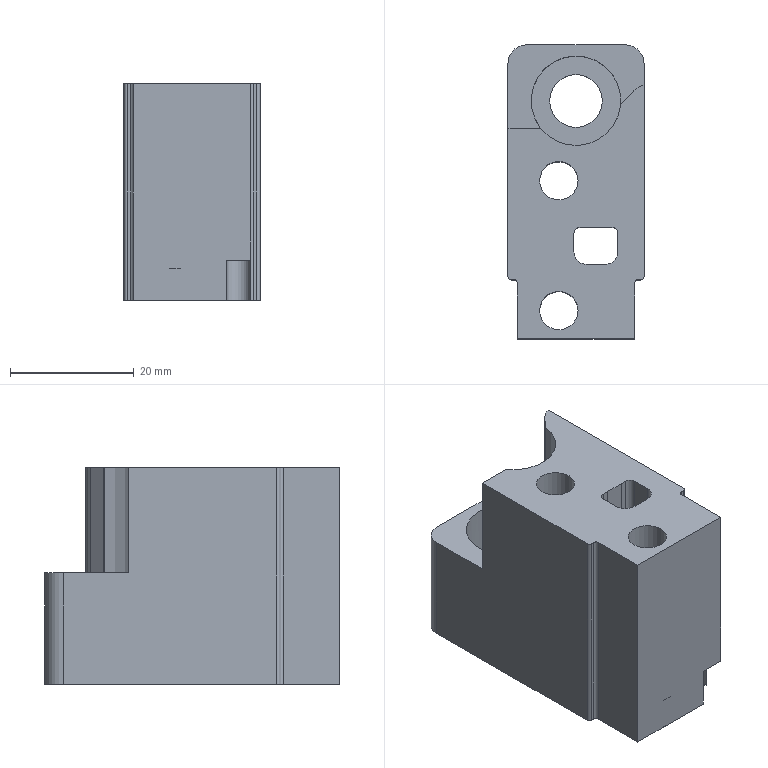Part | NX | features DIE-98 2 | 1 solid | 47 faces | box 22 x 47.549 x 35 mm | volume 24498 mm3 | plane 26 | cylinder 21 | commonest cylinder face diameters 6 x5 1 x4 4 x3 2 x2 6.2 x2 9 x2
STEP:
#1=CARTESIAN_POINT('',(4181.287,-820.122,858.716));
#2=VERTEX_POINT('',#1);
#3=CARTESIAN_POINT('',(4194.237,-816.266,858.716));
#4=VERTEX_POINT('',#3);
#5=CARTESIAN_POINT('',(4187.011,-815.672,858.716));
#6=DIRECTION('',(0.,0.,1.));
#7=DIRECTION('',(1.,0.,0.));
#8=AXIS2_PLACEMENT_3D('',#5,#6,#7);
#9=CIRCLE('',#8,7.25);
#10=EDGE_CURVE('',#2,#4,#9,.T.);
#11=ORIENTED_EDGE('',*,*,#10,.F.);
#12=CARTESIAN_POINT('',(4176.011,-820.122,858.716));
#13=VERTEX_POINT('',#12);
#14=CARTESIAN_POINT('',(3445.094,-820.122,858.716));
#15=DIRECTION('',(-1.,0.,0.));
#16=VECTOR('',#15,1000.);
#17=LINE('',#14,#16);
#18=EDGE_CURVE('',#2,#13,#17,.T.);
#19=ORIENTED_EDGE('',*,*,#18,.T.);
#20=CARTESIAN_POINT('',(4176.011,-844.123,858.716));
#21=VERTEX_POINT('',#20);
#22=CARTESIAN_POINT('',(4176.011,-999.122,858.716));
#23=DIRECTION('',(0.,-1.,0.));
#24=VECTOR('',#23,1000.);
#25=LINE('',#22,#24);
#26=EDGE_CURVE('',#13,#21,#25,.T.);
#27=ORIENTED_EDGE('',*,*,#26,.T.);
#28=CARTESIAN_POINT('',(4176.511,-844.623,858.716));
#29=VERTEX_POINT('',#28);
#30=CARTESIAN_POINT('',(4176.511,-844.123,858.716));
#31=DIRECTION('',(0.,0.,1.));
#32=DIRECTION('',(1.,0.,0.));
#33=AXIS2_PLACEMENT_3D('',#30,#31,#32);
#34=CIRCLE('',#33,0.5);
#35=EDGE_CURVE('',#21,#29,#34,.T.);
#36=ORIENTED_EDGE('',*,*,#35,.T.);
#37=CARTESIAN_POINT('',(4177.011,-844.623,858.716));
#38=VERTEX_POINT('',#37);
#39=CARTESIAN_POINT('',(3445.094,-844.623,858.716));
#40=DIRECTION('',(-1.,0.,0.));
#41=VECTOR('',#40,1000.);
#42=LINE('',#39,#41);
#43=EDGE_CURVE('',#29,#38,#42,.F.);
#44=ORIENTED_EDGE('',*,*,#43,.T.);
#45=CARTESIAN_POINT('',(4177.511,-845.123,858.716));
#46=VERTEX_POINT('',#45);
#47=CARTESIAN_POINT('',(4177.011,-845.123,858.716));
#48=DIRECTION('',(0.,0.,1.));
#49=DIRECTION('',(1.,0.,0.));
#50=AXIS2_PLACEMENT_3D('',#47,#48,#49);
#51=CIRCLE('',#50,0.5);
#52=EDGE_CURVE('',#38,#46,#51,.F.);
#53=ORIENTED_EDGE('',*,*,#52,.T.);
#54=CARTESIAN_POINT('',(4177.511,-854.172,858.716));
#55=VERTEX_POINT('',#54);
#56=CARTESIAN_POINT('',(4177.511,-839.123,858.716));
#57=DIRECTION('',(0.,-1.,0.));
#58=VECTOR('',#57,1000.);
#59=LINE('',#56,#58);
#60=EDGE_CURVE('',#46,#55,#59,.T.);
#61=ORIENTED_EDGE('',*,*,#60,.T.);
#62=CARTESIAN_POINT('',(4196.511,-854.172,858.716));
#63=VERTEX_POINT('',#62);
#64=CARTESIAN_POINT('',(4199.495,-854.172,858.716));
#65=DIRECTION('',(-1.,0.,0.));
#66=VECTOR('',#65,1000.);
#67=LINE('',#64,#66);
#68=EDGE_CURVE('',#63,#55,#67,.T.);
#69=ORIENTED_EDGE('',*,*,#68,.F.);
#70=CARTESIAN_POINT('',(4196.511,-845.123,858.716));
#71=VERTEX_POINT('',#70);
#72=CARTESIAN_POINT('',(4196.511,-839.123,858.716));
#73=DIRECTION('',(0.,1.,0.));
#74=VECTOR('',#73,1000.);
#75=LINE('',#72,#74);
#76=EDGE_CURVE('',#71,#63,#75,.F.);
#77=ORIENTED_EDGE('',*,*,#76,.F.);
#78=CARTESIAN_POINT('',(4197.011,-844.623,858.716));
#79=VERTEX_POINT('',#78);
#80=CARTESIAN_POINT('',(4197.011,-845.123,858.716));
#81=DIRECTION('',(0.,0.,1.));
#82=DIRECTION('',(1.,0.,0.));
#83=AXIS2_PLACEMENT_3D('',#80,#81,#82);
#84=CIRCLE('',#83,0.5);
#85=EDGE_CURVE('',#71,#79,#84,.F.);
#86=ORIENTED_EDGE('',*,*,#85,.T.);
#87=CARTESIAN_POINT('',(4197.511,-844.623,858.716));
#88=VERTEX_POINT('',#87);
#89=CARTESIAN_POINT('',(3445.094,-844.623,858.716));
#90=DIRECTION('',(-1.,0.,0.));
#91=VECTOR('',#90,1000.);
#92=LINE('',#89,#91);
#93=EDGE_CURVE('',#79,#88,#92,.F.);
#94=ORIENTED_EDGE('',*,*,#93,.T.);
#95=CARTESIAN_POINT('',(4198.011,-844.123,858.716));
#96=VERTEX_POINT('',#95);
#97=CARTESIAN_POINT('',(4197.511,-844.123,858.716));
#98=DIRECTION('',(0.,0.,1.));
#99=DIRECTION('',(1.,0.,0.));
#100=AXIS2_PLACEMENT_3D('',#97,#98,#99);
#101=CIRCLE('',#100,0.5);
#102=EDGE_CURVE('',#88,#96,#101,.T.);
#103=ORIENTED_EDGE('',*,*,#102,.T.);
#104=CARTESIAN_POINT('',(4198.011,-813.17,858.716));
#105=VERTEX_POINT('',#104);
#106=CARTESIAN_POINT('',(4198.011,-839.123,858.716));
#107=DIRECTION('',(0.,-1.,0.));
#108=VECTOR('',#107,1000.);
#109=LINE('',#106,#108);
#110=EDGE_CURVE('',#105,#96,#109,.T.);
#111=ORIENTED_EDGE('',*,*,#110,.F.);
#112=CARTESIAN_POINT('',(4196.39,-814.038,858.716));
#113=VERTEX_POINT('',#112);
#114=CARTESIAN_POINT('',(4198.548,-816.122,858.716));
#115=DIRECTION('',(0.,0.,1.));
#116=DIRECTION('',(1.,0.,0.));
#117=AXIS2_PLACEMENT_3D('',#114,#115,#116);
#118=CIRCLE('',#117,3.);
#119=EDGE_CURVE('',#113,#105,#118,.F.);
#120=ORIENTED_EDGE('',*,*,#119,.F.);
#121=CARTESIAN_POINT('',(4194.348,-816.153,858.716));
#122=VERTEX_POINT('',#121);
#123=CARTESIAN_POINT('',(3741.364,-1285.228,858.716));
#124=DIRECTION('',(-0.6947,-0.7193,0.));
#125=VECTOR('',#124,1000.);
#126=LINE('',#123,#125);
#127=EDGE_CURVE('',#113,#122,#126,.T.);
#128=ORIENTED_EDGE('',*,*,#127,.T.);
#129=CARTESIAN_POINT('',(4184.996,-807.122,858.716));
#130=DIRECTION('',(0.,0.,1.));
#131=DIRECTION('',(1.,0.,0.));
#132=AXIS2_PLACEMENT_3D('',#129,#130,#131);
#133=CIRCLE('',#132,13.);
#134=EDGE_CURVE('',#4,#122,#133,.T.);
#135=ORIENTED_EDGE('',*,*,#134,.F.);
#136=EDGE_LOOP('',(#11,#19,#27,#36,#44,#53,#61,#69,#77,#86,#94,#103,#111,#120,#128,#135));
#137=FACE_BOUND('',#136,.T.);
#138=CARTESIAN_POINT('',(4193.786,-837.122,858.716));
#139=VERTEX_POINT('',#138);
#140=CARTESIAN_POINT('',(4193.786,-840.122,858.716));
#141=VERTEX_POINT('',#140);
#142=CARTESIAN_POINT('',(4193.786,-839.122,858.716));
#143=DIRECTION('',(0.,-1.,0.));
#144=VECTOR('',#143,1000.);
#145=LINE('',#142,#144);
#146=EDGE_CURVE('',#139,#141,#145,.T.);
#147=ORIENTED_EDGE('',*,*,#146,.T.);
#148=CARTESIAN_POINT('',(4191.786,-842.122,858.716));
#149=VERTEX_POINT('',#148);
#150=CARTESIAN_POINT('',(4191.786,-840.122,858.716));
#151=DIRECTION('',(0.,0.,1.));
#152=DIRECTION('',(1.,0.,0.));
#153=AXIS2_PLACEMENT_3D('',#150,#151,#152);
#154=CIRCLE('',#153,2.);
#155=EDGE_CURVE('',#149,#141,#154,.T.);
#156=ORIENTED_EDGE('',*,*,#155,.F.);
#157=CARTESIAN_POINT('',(4188.686,-842.122,858.716));
#158=VERTEX_POINT('',#157);
#159=CARTESIAN_POINT('',(3445.094,-842.122,858.716));
#160=DIRECTION('',(1.,0.,0.));
#161=VECTOR('',#160,1000.);
#162=LINE('',#159,#161);
#163=EDGE_CURVE('',#158,#149,#162,.T.);
#164=ORIENTED_EDGE('',*,*,#163,.F.);
#165=CARTESIAN_POINT('',(4186.686,-840.122,858.716));
#166=VERTEX_POINT('',#165);
#167=CARTESIAN_POINT('',(4188.686,-840.122,858.716));
#168=DIRECTION('',(0.,0.,1.));
#169=DIRECTION('',(1.,0.,0.));
#170=AXIS2_PLACEMENT_3D('',#167,#168,#169);
#171=CIRCLE('',#170,2.);
#172=EDGE_CURVE('',#166,#158,#171,.T.);
#173=ORIENTED_EDGE('',*,*,#172,.F.);
#174=CARTESIAN_POINT('',(4186.686,-837.122,858.716));
#175=VERTEX_POINT('',#174);
#176=CARTESIAN_POINT('',(4186.686,-839.122,858.716));
#177=DIRECTION('',(0.,1.,0.));
#178=VECTOR('',#177,1000.);
#179=LINE('',#176,#178);
#180=EDGE_CURVE('',#166,#175,#179,.T.);
#181=ORIENTED_EDGE('',*,*,#180,.T.);
#182=CARTESIAN_POINT('',(4187.686,-836.122,858.716));
#183=VERTEX_POINT('',#182);
#184=CARTESIAN_POINT('',(4187.686,-837.122,858.716));
#185=DIRECTION('',(0.,0.,1.));
#186=DIRECTION('',(1.,0.,0.));
#187=AXIS2_PLACEMENT_3D('',#184,#185,#186);
#188=CIRCLE('',#187,1.);
#189=EDGE_CURVE('',#175,#183,#188,.F.);
#190=ORIENTED_EDGE('',*,*,#189,.T.);
#191=CARTESIAN_POINT('',(4188.686,-836.122,858.716));
#192=VERTEX_POINT('',#191);
#193=CARTESIAN_POINT('',(4190.736,-836.122,858.716));
#194=DIRECTION('',(1.,0.,0.));
#195=VECTOR('',#194,1000.);
#196=LINE('',#193,#195);
#197=EDGE_CURVE('',#183,#192,#196,.T.);
#198=ORIENTED_EDGE('',*,*,#197,.T.);
#199=CARTESIAN_POINT('',(4191.786,-836.122,858.716));
#200=VERTEX_POINT('',#199);
#201=CARTESIAN_POINT('',(4189.736,-836.122,858.716));
#202=DIRECTION('',(1.,0.,0.));
#203=VECTOR('',#202,1000.);
#204=LINE('',#201,#203);
#205=EDGE_CURVE('',#192,#200,#204,.T.);
#206=ORIENTED_EDGE('',*,*,#205,.T.);
#207=CARTESIAN_POINT('',(4192.786,-836.122,858.716));
#208=VERTEX_POINT('',#207);
#209=CARTESIAN_POINT('',(4190.736,-836.122,858.716));
#210=DIRECTION('',(1.,0.,0.));
#211=VECTOR('',#210,1000.);
#212=LINE('',#209,#211);
#213=EDGE_CURVE('',#200,#208,#212,.T.);
#214=ORIENTED_EDGE('',*,*,#213,.T.);
#215=CARTESIAN_POINT('',(4192.786,-837.122,858.716));
#216=DIRECTION('',(0.,0.,1.));
#217=DIRECTION('',(1.,0.,0.));
#218=AXIS2_PLACEMENT_3D('',#215,#216,#217);
#219=CIRCLE('',#218,1.);
#220=EDGE_CURVE('',#208,#139,#219,.F.);
#221=ORIENTED_EDGE('',*,*,#220,.T.);
#222=EDGE_LOOP('',(#147,#156,#164,#173,#181,#190,#198,#206,#214,#221));
#223=FACE_BOUND('',#222,.T.);
#224=CARTESIAN_POINT('',(4187.336,-828.622,858.716));
#225=VERTEX_POINT('',#224);
#226=CARTESIAN_POINT('',(4184.236,-828.622,858.716));
#227=DIRECTION('',(0.,0.,1.));
#228=DIRECTION('',(1.,0.,0.));
#229=AXIS2_PLACEMENT_3D('',#226,#227,#228);
#230=CIRCLE('',#229,3.1);
#231=EDGE_CURVE('',#225,#225,#230,.F.);
#232=ORIENTED_EDGE('',*,*,#231,.T.);
#233=EDGE_LOOP('',(#232));
#234=FACE_BOUND('',#233,.T.);
#235=CARTESIAN_POINT('',(4187.336,-849.622,858.716));
#236=VERTEX_POINT('',#235);
#237=CARTESIAN_POINT('',(4184.236,-849.622,858.716));
#238=DIRECTION('',(0.,0.,1.));
#239=DIRECTION('',(1.,0.,0.));
#240=AXIS2_PLACEMENT_3D('',#237,#238,#239);
#241=CIRCLE('',#240,3.1);
#242=EDGE_CURVE('',#236,#236,#241,.T.);
#243=ORIENTED_EDGE('',*,*,#242,.F.);
#244=EDGE_LOOP('',(#243));
#245=FACE_BOUND('',#244,.T.);
#246=CARTESIAN_POINT('',(3445.094,-999.122,858.716));
#247=DIRECTION('',(0.,0.,1.));
#248=DIRECTION('',(0.,1.,0.));
#249=AXIS2_PLACEMENT_3D('',#246,#247,#248);
#250=PLANE('',#249);
#251=ADVANCED_FACE('',(#137,#223,#234,#245),#250,.T.);
#252=ORIENTED_EDGE('',*,*,#26,.F.);
#253=CARTESIAN_POINT('',(4176.011,-820.122,841.716));
#254=VERTEX_POINT('',#253);
#255=CARTESIAN_POINT('',(4176.011,-820.122,823.716));
#256=DIRECTION('',(0.,0.,-1.));
#257=VECTOR('',#256,1000.);
#258=LINE('',#255,#257);
#259=EDGE_CURVE('',#13,#254,#258,.T.);
#260=ORIENTED_EDGE('',*,*,#259,.T.);
#261=CARTESIAN_POINT('',(4176.011,-809.623,841.716));
#262=VERTEX_POINT('',#261);
#263=CARTESIAN_POINT('',(4176.011,-813.754,841.716));
#264=DIRECTION('',(0.,1.,0.));
#265=VECTOR('',#264,1000.);
#266=LINE('',#263,#265);
#267=EDGE_CURVE('',#262,#254,#266,.F.);
#268=ORIENTED_EDGE('',*,*,#267,.F.);
#269=CARTESIAN_POINT('',(4176.011,-809.623,823.716));
#270=VERTEX_POINT('',#269);
#271=CARTESIAN_POINT('',(4176.011,-809.623,823.716));
#272=DIRECTION('',(0.,0.,1.));
#273=VECTOR('',#272,1000.);
#274=LINE('',#271,#273);
#275=EDGE_CURVE('',#270,#262,#274,.T.);
#276=ORIENTED_EDGE('',*,*,#275,.F.);
#277=CARTESIAN_POINT('',(4176.011,-844.123,823.716));
#278=VERTEX_POINT('',#277);
#279=CARTESIAN_POINT('',(4176.011,-999.122,823.716));
#280=DIRECTION('',(0.,-1.,0.));
#281=VECTOR('',#280,1000.);
#282=LINE('',#279,#281);
#283=EDGE_CURVE('',#278,#270,#282,.F.);
#284=ORIENTED_EDGE('',*,*,#283,.F.);
#285=CARTESIAN_POINT('',(4176.011,-844.123,823.716));
#286=DIRECTION('',(0.,0.,1.));
#287=VECTOR('',#286,1000.);
#288=LINE('',#285,#287);
#289=EDGE_CURVE('',#278,#21,#288,.T.);
#290=ORIENTED_EDGE('',*,*,#289,.T.);
#291=EDGE_LOOP('',(#252,#260,#268,#276,#284,#290));
#292=FACE_BOUND('',#291,.T.);
#293=CARTESIAN_POINT('',(4176.011,-839.123,823.716));
#294=DIRECTION('',(-1.,0.,0.));
#295=DIRECTION('',(0.,0.,1.));
#296=AXIS2_PLACEMENT_3D('',#293,#294,#295);
#297=PLANE('',#296);
#298=ADVANCED_FACE('',(#292),#297,.T.);
#299=CARTESIAN_POINT('',(4191.261,-815.672,823.716));
#300=VERTEX_POINT('',#299);
#301=CARTESIAN_POINT('',(4187.011,-815.672,823.716));
#302=DIRECTION('',(0.,0.,1.));
#303=DIRECTION('',(1.,0.,0.));
#304=AXIS2_PLACEMENT_3D('',#301,#302,#303);
#305=CIRCLE('',#304,4.25);
#306=EDGE_CURVE('',#300,#300,#305,.F.);
#307=ORIENTED_EDGE('',*,*,#306,.F.);
#308=EDGE_LOOP('',(#307));
#309=FACE_BOUND('',#308,.T.);
#310=CARTESIAN_POINT('',(4186.686,-839.69,823.716));
#311=VERTEX_POINT('',#310);
#312=CARTESIAN_POINT('',(4188.236,-834.122,823.716));
#313=VERTEX_POINT('',#312);
#314=CARTESIAN_POINT('',(4188.236,-837.122,823.716));
#315=DIRECTION('',(0.,0.,1.));
#316=DIRECTION('',(1.,0.,0.));
#317=AXIS2_PLACEMENT_3D('',#314,#315,#316);
#318=CIRCLE('',#317,3.);
#319=EDGE_CURVE('',#311,#313,#318,.F.);
#320=ORIENTED_EDGE('',*,*,#319,.F.);
#321=CARTESIAN_POINT('',(4186.686,-840.122,823.716));
#322=VERTEX_POINT('',#321);
#323=CARTESIAN_POINT('',(4186.686,-839.122,823.716));
#324=DIRECTION('',(0.,1.,0.));
#325=VECTOR('',#324,1000.);
#326=LINE('',#323,#325);
#327=EDGE_CURVE('',#311,#322,#326,.F.);
#328=ORIENTED_EDGE('',*,*,#327,.T.);
#329=CARTESIAN_POINT('',(4188.686,-842.122,823.716));
#330=VERTEX_POINT('',#329);
#331=CARTESIAN_POINT('',(4188.686,-840.122,823.716));
#332=DIRECTION('',(0.,0.,1.));
#333=DIRECTION('',(1.,0.,0.));
#334=AXIS2_PLACEMENT_3D('',#331,#332,#333);
#335=CIRCLE('',#334,2.);
#336=EDGE_CURVE('',#330,#322,#335,.F.);
#337=ORIENTED_EDGE('',*,*,#336,.F.);
#338=CARTESIAN_POINT('',(4191.786,-842.122,823.716));
#339=VERTEX_POINT('',#338);
#340=CARTESIAN_POINT('',(3445.094,-842.122,823.716));
#341=DIRECTION('',(1.,0.,0.));
#342=VECTOR('',#341,1000.);
#343=LINE('',#340,#342);
#344=EDGE_CURVE('',#339,#330,#343,.F.);
#345=ORIENTED_EDGE('',*,*,#344,.F.);
#346=CARTESIAN_POINT('',(4193.786,-840.122,823.716));
#347=VERTEX_POINT('',#346);
#348=CARTESIAN_POINT('',(4191.786,-840.122,823.716));
#349=DIRECTION('',(0.,0.,1.));
#350=DIRECTION('',(1.,0.,0.));
#351=AXIS2_PLACEMENT_3D('',#348,#349,#350);
#352=CIRCLE('',#351,2.);
#353=EDGE_CURVE('',#347,#339,#352,.F.);
#354=ORIENTED_EDGE('',*,*,#353,.F.);
#355=CARTESIAN_POINT('',(4193.786,-839.69,823.716));
#356=VERTEX_POINT('',#355);
#357=CARTESIAN_POINT('',(4193.786,-839.122,823.716));
#358=DIRECTION('',(0.,-1.,0.));
#359=VECTOR('',#358,1000.);
#360=LINE('',#357,#359);
#361=EDGE_CURVE('',#347,#356,#360,.F.);
#362=ORIENTED_EDGE('',*,*,#361,.T.);
#363=CARTESIAN_POINT('',(4192.236,-834.122,823.716));
#364=VERTEX_POINT('',#363);
#365=CARTESIAN_POINT('',(4192.236,-837.122,823.716));
#366=DIRECTION('',(0.,0.,1.));
#367=DIRECTION('',(1.,0.,0.));
#368=AXIS2_PLACEMENT_3D('',#365,#366,#367);
#369=CIRCLE('',#368,3.);
#370=EDGE_CURVE('',#364,#356,#369,.F.);
#371=ORIENTED_EDGE('',*,*,#370,.F.);
#372=CARTESIAN_POINT('',(4188.236,-834.122,823.716));
#373=DIRECTION('',(-1.,0.,0.));
#374=VECTOR('',#373,1000.);
#375=LINE('',#372,#374);
#376=EDGE_CURVE('',#313,#364,#375,.F.);
#377=ORIENTED_EDGE('',*,*,#376,.F.);
#378=EDGE_LOOP('',(#320,#328,#337,#345,#354,#362,#371,#377));
#379=FACE_BOUND('',#378,.T.);
#380=CARTESIAN_POINT('',(4188.736,-828.622,823.716));
#381=VERTEX_POINT('',#380);
#382=CARTESIAN_POINT('',(4184.236,-828.622,823.716));
#383=DIRECTION('',(0.,0.,1.));
#384=DIRECTION('',(1.,0.,0.));
#385=AXIS2_PLACEMENT_3D('',#382,#383,#384);
#386=CIRCLE('',#385,4.5);
#387=EDGE_CURVE('',#381,#381,#386,.T.);
#388=ORIENTED_EDGE('',*,*,#387,.T.);
#389=EDGE_LOOP('',(#388));
#390=FACE_BOUND('',#389,.T.);
#391=CARTESIAN_POINT('',(4188.736,-849.622,823.716));
#392=VERTEX_POINT('',#391);
#393=CARTESIAN_POINT('',(4184.236,-849.622,823.716));
#394=DIRECTION('',(0.,0.,1.));
#395=DIRECTION('',(1.,0.,0.));
#396=AXIS2_PLACEMENT_3D('',#393,#394,#395);
#397=CIRCLE('',#396,4.5);
#398=EDGE_CURVE('',#392,#392,#397,.T.);
#399=ORIENTED_EDGE('',*,*,#398,.T.);
#400=EDGE_LOOP('',(#399));
#401=FACE_BOUND('',#400,.T.);
#402=CARTESIAN_POINT('',(4192.535,-851.122,823.716));
#403=VERTEX_POINT('',#402);
#404=CARTESIAN_POINT('',(4196.511,-850.812,823.716));
#405=VERTEX_POINT('',#404);
#406=CARTESIAN_POINT('',(4194.535,-851.122,823.716));
#407=DIRECTION('',(0.,0.,-1.));
#408=DIRECTION('',(1.,0.,0.));
#409=AXIS2_PLACEMENT_3D('',#406,#407,#408);
#410=CIRCLE('',#409,2.);
#411=EDGE_CURVE('',#403,#405,#410,.T.);
#412=ORIENTED_EDGE('',*,*,#411,.F.);
#413=CARTESIAN_POINT('',(4192.535,-854.172,823.716));
#414=VERTEX_POINT('',#413);
#415=CARTESIAN_POINT('',(4192.535,-851.122,823.716));
#416=DIRECTION('',(0.,-1.,0.));
#417=VECTOR('',#416,1000.);
#418=LINE('',#415,#417);
#419=EDGE_CURVE('',#403,#414,#418,.T.);
#420=ORIENTED_EDGE('',*,*,#419,.T.);
#421=CARTESIAN_POINT('',(4177.511,-854.172,823.716));
#422=VERTEX_POINT('',#421);
#423=CARTESIAN_POINT('',(3445.094,-854.172,823.716));
#424=DIRECTION('',(-1.,0.,0.));
#425=VECTOR('',#424,1000.);
#426=LINE('',#423,#425);
#427=EDGE_CURVE('',#422,#414,#426,.F.);
#428=ORIENTED_EDGE('',*,*,#427,.F.);
#429=CARTESIAN_POINT('',(4177.511,-845.123,823.716));
#430=VERTEX_POINT('',#429);
#431=CARTESIAN_POINT('',(4177.511,-839.123,823.716));
#432=DIRECTION('',(0.,1.,0.));
#433=VECTOR('',#432,1000.);
#434=LINE('',#431,#433);
#435=EDGE_CURVE('',#422,#430,#434,.T.);
#436=ORIENTED_EDGE('',*,*,#435,.T.);
#437=CARTESIAN_POINT('',(4177.011,-844.623,823.716));
#438=VERTEX_POINT('',#437);
#439=CARTESIAN_POINT('',(4177.011,-845.123,823.716));
#440=DIRECTION('',(0.,0.,1.));
#441=DIRECTION('',(1.,0.,0.));
#442=AXIS2_PLACEMENT_3D('',#439,#440,#441);
#443=CIRCLE('',#442,0.5);
#444=EDGE_CURVE('',#430,#438,#443,.T.);
#445=ORIENTED_EDGE('',*,*,#444,.T.);
#446=CARTESIAN_POINT('',(4176.511,-844.623,823.716));
#447=VERTEX_POINT('',#446);
#448=CARTESIAN_POINT('',(3445.094,-844.623,823.716));
#449=DIRECTION('',(-1.,0.,0.));
#450=VECTOR('',#449,1000.);
#451=LINE('',#448,#450);
#452=EDGE_CURVE('',#447,#438,#451,.F.);
#453=ORIENTED_EDGE('',*,*,#452,.F.);
#454=CARTESIAN_POINT('',(4176.511,-844.123,823.716));
#455=DIRECTION('',(0.,0.,1.));
#456=DIRECTION('',(1.,0.,0.));
#457=AXIS2_PLACEMENT_3D('',#454,#455,#456);
#458=CIRCLE('',#457,0.5);
#459=EDGE_CURVE('',#447,#278,#458,.F.);
#460=ORIENTED_EDGE('',*,*,#459,.T.);
#461=ORIENTED_EDGE('',*,*,#283,.T.);
#462=CARTESIAN_POINT('',(4179.011,-806.623,823.716));
#463=VERTEX_POINT('',#462);
#464=CARTESIAN_POINT('',(4179.011,-809.623,823.716));
#465=DIRECTION('',(0.,0.,1.));
#466=DIRECTION('',(-1.,0.,0.));
#467=AXIS2_PLACEMENT_3D('',#464,#465,#466);
#468=CIRCLE('',#467,3.);
#469=EDGE_CURVE('',#463,#270,#468,.T.);
#470=ORIENTED_EDGE('',*,*,#469,.F.);
#471=CARTESIAN_POINT('',(4195.011,-806.623,823.716));
#472=VERTEX_POINT('',#471);
#473=CARTESIAN_POINT('',(3445.094,-806.623,823.716));
#474=DIRECTION('',(-1.,0.,0.));
#475=VECTOR('',#474,1000.);
#476=LINE('',#473,#475);
#477=EDGE_CURVE('',#463,#472,#476,.F.);
#478=ORIENTED_EDGE('',*,*,#477,.T.);
#479=CARTESIAN_POINT('',(4198.011,-809.623,823.716));
#480=VERTEX_POINT('',#479);
#481=CARTESIAN_POINT('',(4195.011,-809.623,823.716));
#482=DIRECTION('',(0.,0.,1.));
#483=DIRECTION('',(-1.,0.,0.));
#484=AXIS2_PLACEMENT_3D('',#481,#482,#483);
#485=CIRCLE('',#484,3.);
#486=EDGE_CURVE('',#480,#472,#485,.T.);
#487=ORIENTED_EDGE('',*,*,#486,.F.);
#488=CARTESIAN_POINT('',(4198.011,-844.123,823.716));
#489=VERTEX_POINT('',#488);
#490=CARTESIAN_POINT('',(4198.011,-999.122,823.716));
#491=DIRECTION('',(0.,1.,0.));
#492=VECTOR('',#491,1000.);
#493=LINE('',#490,#492);
#494=EDGE_CURVE('',#480,#489,#493,.F.);
#495=ORIENTED_EDGE('',*,*,#494,.T.);
#496=CARTESIAN_POINT('',(4197.511,-844.623,823.716));
#497=VERTEX_POINT('',#496);
#498=CARTESIAN_POINT('',(4197.511,-844.123,823.716));
#499=DIRECTION('',(0.,0.,1.));
#500=DIRECTION('',(1.,0.,0.));
#501=AXIS2_PLACEMENT_3D('',#498,#499,#500);
#502=CIRCLE('',#501,0.5);
#503=EDGE_CURVE('',#489,#497,#502,.F.);
#504=ORIENTED_EDGE('',*,*,#503,.T.);
#505=CARTESIAN_POINT('',(4197.011,-844.623,823.716));
#506=VERTEX_POINT('',#505);
#507=CARTESIAN_POINT('',(3445.094,-844.623,823.716));
#508=DIRECTION('',(-1.,0.,0.));
#509=VECTOR('',#508,1000.);
#510=LINE('',#507,#509);
#511=EDGE_CURVE('',#506,#497,#510,.F.);
#512=ORIENTED_EDGE('',*,*,#511,.F.);
#513=CARTESIAN_POINT('',(4196.511,-845.123,823.716));
#514=VERTEX_POINT('',#513);
#515=CARTESIAN_POINT('',(4197.011,-845.123,823.716));
#516=DIRECTION('',(0.,0.,1.));
#517=DIRECTION('',(1.,0.,0.));
#518=AXIS2_PLACEMENT_3D('',#515,#516,#517);
#519=CIRCLE('',#518,0.5);
#520=EDGE_CURVE('',#506,#514,#519,.T.);
#521=ORIENTED_EDGE('',*,*,#520,.T.);
#522=CARTESIAN_POINT('',(4196.511,-839.123,823.716));
#523=DIRECTION('',(0.,-1.,0.));
#524=VECTOR('',#523,1000.);
#525=LINE('',#522,#524);
#526=EDGE_CURVE('',#514,#405,#525,.T.);
#527=ORIENTED_EDGE('',*,*,#526,.T.);
#528=EDGE_LOOP('',(#412,#420,#428,#436,#445,#453,#460,#461,#470,#478,#487,#495,#504,#512,#521,#527));
#529=FACE_BOUND('',#528,.T.);
#530=CARTESIAN_POINT('',(3445.094,-999.122,823.716));
#531=DIRECTION('',(0.,0.,1.));
#532=DIRECTION('',(0.,1.,0.));
#533=AXIS2_PLACEMENT_3D('',#530,#531,#532);
#534=PLANE('',#533);
#535=ADVANCED_FACE('',(#309,#379,#390,#401,#529),#534,.F.);
#536=CARTESIAN_POINT('',(4192.535,-854.172,830.216));
#537=VERTEX_POINT('',#536);
#538=CARTESIAN_POINT('',(4192.535,-854.172,858.716));
#539=DIRECTION('',(0.,0.,-1.));
#540=VECTOR('',#539,1000.);
#541=LINE('',#538,#540);
#542=EDGE_CURVE('',#537,#414,#541,.T.);
#543=ORIENTED_EDGE('',*,*,#542,.F.);
#544=CARTESIAN_POINT('',(4196.511,-854.172,830.216));
#545=VERTEX_POINT('',#544);
#546=CARTESIAN_POINT('',(4199.495,-854.172,830.216));
#547=DIRECTION('',(-1.,0.,0.));
#548=VECTOR('',#547,1000.);
#549=LINE('',#546,#548);
#550=EDGE_CURVE('',#545,#537,#549,.T.);
#551=ORIENTED_EDGE('',*,*,#550,.F.);
#552=CARTESIAN_POINT('',(4196.511,-854.172,858.716));
#553=DIRECTION('',(0.,0.,-1.));
#554=VECTOR('',#553,1000.);
#555=LINE('',#552,#554);
#556=EDGE_CURVE('',#63,#545,#555,.T.);
#557=ORIENTED_EDGE('',*,*,#556,.F.);
#558=ORIENTED_EDGE('',*,*,#68,.T.);
#559=CARTESIAN_POINT('',(4177.511,-854.172,823.716));
#560=DIRECTION('',(0.,0.,-1.));
#561=VECTOR('',#560,1000.);
#562=LINE('',#559,#561);
#563=EDGE_CURVE('',#55,#422,#562,.T.);
#564=ORIENTED_EDGE('',*,*,#563,.T.);
#565=ORIENTED_EDGE('',*,*,#427,.T.);
#566=EDGE_LOOP('',(#543,#551,#557,#558,#564,#565));
#567=FACE_BOUND('',#566,.T.);
#568=CARTESIAN_POINT('',(4199.495,-854.172,858.716));
#569=DIRECTION('',(0.,1.,0.));
#570=DIRECTION('',(-1.,0.,0.));
#571=AXIS2_PLACEMENT_3D('',#568,#569,#570);
#572=PLANE('',#571);
#573=ADVANCED_FACE('',(#567),#572,.F.);
#574=ORIENTED_EDGE('',*,*,#511,.T.);
#575=CARTESIAN_POINT('',(4197.511,-844.623,858.716));
#576=DIRECTION('',(0.,0.,-1.));
#577=VECTOR('',#576,1000.);
#578=LINE('',#575,#577);
#579=EDGE_CURVE('',#497,#88,#578,.F.);
#580=ORIENTED_EDGE('',*,*,#579,.T.);
#581=ORIENTED_EDGE('',*,*,#93,.F.);
#582=CARTESIAN_POINT('',(4197.011,-844.623,841.216));
#583=DIRECTION('',(0.,0.,1.));
#584=VECTOR('',#583,1000.);
#585=LINE('',#582,#584);
#586=EDGE_CURVE('',#79,#506,#585,.F.);
#587=ORIENTED_EDGE('',*,*,#586,.T.);
#588=EDGE_LOOP('',(#574,#580,#581,#587));
#589=FACE_BOUND('',#588,.T.);
#590=CARTESIAN_POINT('',(4187.011,-844.623,841.216));
#591=DIRECTION('',(0.,1.,0.));
#592=DIRECTION('',(0.,0.,1.));
#593=AXIS2_PLACEMENT_3D('',#590,#591,#592);
#594=PLANE('',#593);
#595=ADVANCED_FACE('',(#589),#594,.F.);
#596=ORIENTED_EDGE('',*,*,#452,.T.);
#597=CARTESIAN_POINT('',(4177.011,-844.623,841.216));
#598=DIRECTION('',(0.,0.,-1.));
#599=VECTOR('',#598,1000.);
#600=LINE('',#597,#599);
#601=EDGE_CURVE('',#438,#38,#600,.F.);
#602=ORIENTED_EDGE('',*,*,#601,.T.);
#603=ORIENTED_EDGE('',*,*,#43,.F.);
#604=CARTESIAN_POINT('',(4176.511,-844.623,823.716));
#605=DIRECTION('',(0.,0.,1.));
#606=VECTOR('',#605,1000.);
#607=LINE('',#604,#606);
#608=EDGE_CURVE('',#29,#447,#607,.F.);
#609=ORIENTED_EDGE('',*,*,#608,.T.);
#610=EDGE_LOOP('',(#596,#602,#603,#609));
#611=FACE_BOUND('',#610,.T.);
#612=CARTESIAN_POINT('',(4187.011,-844.623,841.216));
#613=DIRECTION('',(0.,1.,0.));
#614=DIRECTION('',(0.,0.,1.));
#615=AXIS2_PLACEMENT_3D('',#612,#613,#614);
#616=PLANE('',#615);
#617=ADVANCED_FACE('',(#611),#616,.F.);
#618=CARTESIAN_POINT('',(4181.136,-828.622,828.916));
#619=VERTEX_POINT('',#618);
#620=CARTESIAN_POINT('',(4184.236,-828.622,828.916));
#621=DIRECTION('',(0.,0.,-1.));
#622=DIRECTION('',(-1.,0.,0.));
#623=AXIS2_PLACEMENT_3D('',#620,#621,#622);
#624=CIRCLE('',#623,3.1);
#625=EDGE_CURVE('',#619,#619,#624,.T.);
#626=ORIENTED_EDGE('',*,*,#625,.F.);
#627=EDGE_LOOP('',(#626));
#628=FACE_BOUND('',#627,.T.);
#629=CARTESIAN_POINT('',(4179.736,-828.622,828.916));
#630=VERTEX_POINT('',#629);
#631=CARTESIAN_POINT('',(4184.236,-828.622,828.916));
#632=DIRECTION('',(0.,0.,-1.));
#633=DIRECTION('',(-1.,0.,0.));
#634=AXIS2_PLACEMENT_3D('',#631,#632,#633);
#635=CIRCLE('',#634,4.5);
#636=EDGE_CURVE('',#630,#630,#635,.F.);
#637=ORIENTED_EDGE('',*,*,#636,.F.);
#638=EDGE_LOOP('',(#637));
#639=FACE_BOUND('',#638,.T.);
#640=CARTESIAN_POINT('',(4217.236,-877.122,828.916));
#641=DIRECTION('',(0.,0.,-1.));
#642=DIRECTION('',(-1.,0.,0.));
#643=AXIS2_PLACEMENT_3D('',#640,#641,#642);
#644=PLANE('',#643);
#645=ADVANCED_FACE('',(#628,#639),#644,.T.);
#646=CARTESIAN_POINT('',(4186.686,-839.69,828.916));
#647=VERTEX_POINT('',#646);
#648=CARTESIAN_POINT('',(4186.686,-837.122,828.916));
#649=VERTEX_POINT('',#648);
#650=CARTESIAN_POINT('',(4186.686,-1716.244,828.916));
#651=DIRECTION('',(0.,1.,0.));
#652=VECTOR('',#651,1000.);
#653=LINE('',#650,#652);
#654=EDGE_CURVE('',#647,#649,#653,.T.);
#655=ORIENTED_EDGE('',*,*,#654,.F.);
#656=CARTESIAN_POINT('',(4188.236,-834.122,828.916));
#657=VERTEX_POINT('',#656);
#658=CARTESIAN_POINT('',(4188.236,-837.122,828.916));
#659=DIRECTION('',(0.,0.,-1.));
#660=DIRECTION('',(-1.,0.,0.));
#661=AXIS2_PLACEMENT_3D('',#658,#659,#660);
#662=CIRCLE('',#661,3.);
#663=EDGE_CURVE('',#647,#657,#662,.T.);
#664=ORIENTED_EDGE('',*,*,#663,.T.);
#665=CARTESIAN_POINT('',(4192.236,-834.122,828.916));
#666=VERTEX_POINT('',#665);
#667=CARTESIAN_POINT('',(4188.236,-834.122,828.916));
#668=DIRECTION('',(1.,0.,0.));
#669=VECTOR('',#668,1000.);
#670=LINE('',#667,#669);
#671=EDGE_CURVE('',#657,#666,#670,.T.);
#672=ORIENTED_EDGE('',*,*,#671,.T.);
#673=CARTESIAN_POINT('',(4193.786,-839.69,828.916));
#674=VERTEX_POINT('',#673);
#675=CARTESIAN_POINT('',(4192.236,-837.122,828.916));
#676=DIRECTION('',(0.,0.,-1.));
#677=DIRECTION('',(-1.,0.,0.));
#678=AXIS2_PLACEMENT_3D('',#675,#676,#677);
#679=CIRCLE('',#678,3.);
#680=EDGE_CURVE('',#666,#674,#679,.T.);
#681=ORIENTED_EDGE('',*,*,#680,.T.);
#682=CARTESIAN_POINT('',(4193.786,-837.122,828.916));
#683=VERTEX_POINT('',#682);
#684=CARTESIAN_POINT('',(4193.786,-1716.244,828.916));
#685=DIRECTION('',(0.,-1.,0.));
#686=VECTOR('',#685,1000.);
#687=LINE('',#684,#686);
#688=EDGE_CURVE('',#683,#674,#687,.T.);
#689=ORIENTED_EDGE('',*,*,#688,.F.);
#690=CARTESIAN_POINT('',(4192.786,-836.122,828.916));
#691=VERTEX_POINT('',#690);
#692=CARTESIAN_POINT('',(4192.786,-837.122,828.916));
#693=DIRECTION('',(0.,0.,-1.));
#694=DIRECTION('',(-1.,0.,0.));
#695=AXIS2_PLACEMENT_3D('',#692,#693,#694);
#696=CIRCLE('',#695,1.);
#697=EDGE_CURVE('',#691,#683,#696,.T.);
#698=ORIENTED_EDGE('',*,*,#697,.F.);
#699=CARTESIAN_POINT('',(4192.236,-836.122,828.916));
#700=VERTEX_POINT('',#699);
#701=CARTESIAN_POINT('',(4190.736,-836.122,828.916));
#702=DIRECTION('',(-1.,0.,0.));
#703=VECTOR('',#702,1000.);
#704=LINE('',#701,#703);
#705=EDGE_CURVE('',#691,#700,#704,.T.);
#706=ORIENTED_EDGE('',*,*,#705,.T.);
#707=CARTESIAN_POINT('',(4191.786,-836.122,828.916));
#708=VERTEX_POINT('',#707);
#709=CARTESIAN_POINT('',(4190.736,-836.122,828.916));
#710=DIRECTION('',(-1.,0.,0.));
#711=VECTOR('',#710,1000.);
#712=LINE('',#709,#711);
#713=EDGE_CURVE('',#700,#708,#712,.T.);
#714=ORIENTED_EDGE('',*,*,#713,.T.);
#715=CARTESIAN_POINT('',(4188.686,-836.122,828.916));
#716=VERTEX_POINT('',#715);
#717=CARTESIAN_POINT('',(0.000000109,-836.122,828.916));
#718=DIRECTION('',(1.,0.,0.));
#719=VECTOR('',#718,1000.);
#720=LINE('',#717,#719);
#721=EDGE_CURVE('',#716,#708,#720,.T.);
#722=ORIENTED_EDGE('',*,*,#721,.F.);
#723=CARTESIAN_POINT('',(4188.236,-836.122,828.916));
#724=VERTEX_POINT('',#723);
#725=CARTESIAN_POINT('',(4190.736,-836.122,828.916));
#726=DIRECTION('',(-1.,0.,0.));
#727=VECTOR('',#726,1000.);
#728=LINE('',#725,#727);
#729=EDGE_CURVE('',#716,#724,#728,.T.);
#730=ORIENTED_EDGE('',*,*,#729,.T.);
#731=CARTESIAN_POINT('',(4187.686,-836.122,828.916));
#732=VERTEX_POINT('',#731);
#733=CARTESIAN_POINT('',(4190.736,-836.122,828.916));
#734=DIRECTION('',(-1.,0.,0.));
#735=VECTOR('',#734,1000.);
#736=LINE('',#733,#735);
#737=EDGE_CURVE('',#724,#732,#736,.T.);
#738=ORIENTED_EDGE('',*,*,#737,.T.);
#739=CARTESIAN_POINT('',(4187.686,-837.122,828.916));
#740=DIRECTION('',(0.,0.,-1.));
#741=DIRECTION('',(-1.,0.,0.));
#742=AXIS2_PLACEMENT_3D('',#739,#740,#741);
#743=CIRCLE('',#742,1.);
#744=EDGE_CURVE('',#649,#732,#743,.T.);
#745=ORIENTED_EDGE('',*,*,#744,.F.);
#746=EDGE_LOOP('',(#655,#664,#672,#681,#689,#698,#706,#714,#722,#730,#738,#745));
#747=FACE_BOUND('',#746,.T.);
#748=CARTESIAN_POINT('',(0.000000011,-1716.244,828.916));
#749=DIRECTION('',(0.,0.,-1.));
#750=DIRECTION('',(-1.,0.,0.));
#751=AXIS2_PLACEMENT_3D('',#748,#749,#750);
#752=PLANE('',#751);
#753=ADVANCED_FACE('',(#747),#752,.T.);
#754=ORIENTED_EDGE('',*,*,#231,.F.);
#755=EDGE_LOOP('',(#754));
#756=FACE_BOUND('',#755,.T.);
#757=ORIENTED_EDGE('',*,*,#625,.T.);
#758=EDGE_LOOP('',(#757));
#759=FACE_BOUND('',#758,.T.);
#760=CARTESIAN_POINT('',(4184.236,-828.622,823.716));
#761=DIRECTION('',(0.,0.,1.));
#762=DIRECTION('',(1.,0.,0.));
#763=AXIS2_PLACEMENT_3D('',#760,#761,#762);
#764=CYLINDRICAL_SURFACE('',#763,3.1);
#765=ADVANCED_FACE('',(#756,#759),#764,.F.);
#766=CARTESIAN_POINT('',(4192.786,-836.122,823.716));
#767=DIRECTION('',(0.,0.,1.));
#768=VECTOR('',#767,1000.);
#769=LINE('',#766,#768);
#770=EDGE_CURVE('',#208,#691,#769,.F.);
#771=ORIENTED_EDGE('',*,*,#770,.T.);
#772=ORIENTED_EDGE('',*,*,#697,.T.);
#773=CARTESIAN_POINT('',(4193.786,-837.122,823.716));
#774=DIRECTION('',(0.,0.,1.));
#775=VECTOR('',#774,1000.);
#776=LINE('',#773,#775);
#777=EDGE_CURVE('',#139,#683,#776,.F.);
#778=ORIENTED_EDGE('',*,*,#777,.F.);
#779=ORIENTED_EDGE('',*,*,#220,.F.);
#780=EDGE_LOOP('',(#771,#772,#778,#779));
#781=FACE_BOUND('',#780,.T.);
#782=CARTESIAN_POINT('',(4192.786,-837.122,823.716));
#783=DIRECTION('',(0.,0.,1.));
#784=DIRECTION('',(1.,0.,0.));
#785=AXIS2_PLACEMENT_3D('',#782,#783,#784);
#786=CYLINDRICAL_SURFACE('',#785,1.);
#787=ADVANCED_FACE('',(#781),#786,.F.);
#788=ORIENTED_EDGE('',*,*,#713,.F.);
#789=ORIENTED_EDGE('',*,*,#705,.F.);
#790=ORIENTED_EDGE('',*,*,#770,.F.);
#791=ORIENTED_EDGE('',*,*,#213,.F.);
#792=CARTESIAN_POINT('',(4191.786,-836.122,828.916));
#793=CARTESIAN_POINT('',(4191.786,-836.122,838.85));
#794=CARTESIAN_POINT('',(4191.786,-836.122,848.783));
#795=CARTESIAN_POINT('',(4191.786,-836.122,858.716));
#796=B_SPLINE_CURVE_WITH_KNOTS('',3,(#792,#793,#794,#795),.UNSPECIFIED.,.F.,.F.,(4,4),(0.006667,1.),.UNSPECIFIED.);
#797=EDGE_CURVE('',#708,#200,#796,.T.);
#798=ORIENTED_EDGE('',*,*,#797,.F.);
#799=EDGE_LOOP('',(#788,#789,#790,#791,#798));
#800=FACE_BOUND('',#799,.T.);
#801=CARTESIAN_POINT('',(4190.736,-836.122,823.716));
#802=DIRECTION('',(0.,1.,0.));
#803=DIRECTION('',(1.,0.,0.));
#804=AXIS2_PLACEMENT_3D('',#801,#802,#803);
#805=PLANE('',#804);
#806=ADVANCED_FACE('',(#800),#805,.F.);
#807=CARTESIAN_POINT('',(4188.686,-836.122,858.716));
#808=CARTESIAN_POINT('',(4188.686,-836.122,848.783));
#809=CARTESIAN_POINT('',(4188.686,-836.122,838.85));
#810=CARTESIAN_POINT('',(4188.686,-836.122,828.916));
#811=B_SPLINE_CURVE_WITH_KNOTS('',3,(#807,#808,#809,#810),.UNSPECIFIED.,.F.,.F.,(4,4),(0.000000025,0.8514),.UNSPECIFIED.);
#812=EDGE_CURVE('',#192,#716,#811,.T.);
#813=ORIENTED_EDGE('',*,*,#812,.T.);
#814=ORIENTED_EDGE('',*,*,#721,.T.);
#815=ORIENTED_EDGE('',*,*,#797,.T.);
#816=ORIENTED_EDGE('',*,*,#205,.F.);
#817=EDGE_LOOP('',(#813,#814,#815,#816));
#818=FACE_BOUND('',#817,.T.);
#819=CARTESIAN_POINT('',(4189.736,-836.122,823.716));
#820=DIRECTION('',(0.,1.,0.));
#821=DIRECTION('',(-1.,0.,0.));
#822=AXIS2_PLACEMENT_3D('',#819,#820,#821);
#823=PLANE('',#822);
#824=ADVANCED_FACE('',(#818),#823,.F.);
#825=CARTESIAN_POINT('',(4187.686,-836.122,823.716));
#826=DIRECTION('',(0.,0.,1.));
#827=VECTOR('',#826,1000.);
#828=LINE('',#825,#827);
#829=EDGE_CURVE('',#732,#183,#828,.T.);
#830=ORIENTED_EDGE('',*,*,#829,.F.);
#831=ORIENTED_EDGE('',*,*,#737,.F.);
#832=ORIENTED_EDGE('',*,*,#729,.F.);
#833=ORIENTED_EDGE('',*,*,#812,.F.);
#834=ORIENTED_EDGE('',*,*,#197,.F.);
#835=EDGE_LOOP('',(#830,#831,#832,#833,#834));
#836=FACE_BOUND('',#835,.T.);
#837=CARTESIAN_POINT('',(4190.736,-836.122,823.716));
#838=DIRECTION('',(0.,1.,0.));
#839=DIRECTION('',(1.,0.,0.));
#840=AXIS2_PLACEMENT_3D('',#837,#838,#839);
#841=PLANE('',#840);
#842=ADVANCED_FACE('',(#836),#841,.F.);
#843=CARTESIAN_POINT('',(4186.686,-837.122,823.716));
#844=DIRECTION('',(0.,0.,1.));
#845=VECTOR('',#844,1000.);
#846=LINE('',#843,#845);
#847=EDGE_CURVE('',#649,#175,#846,.T.);
#848=ORIENTED_EDGE('',*,*,#847,.F.);
#849=ORIENTED_EDGE('',*,*,#744,.T.);
#850=ORIENTED_EDGE('',*,*,#829,.T.);
#851=ORIENTED_EDGE('',*,*,#189,.F.);
#852=EDGE_LOOP('',(#848,#849,#850,#851));
#853=FACE_BOUND('',#852,.T.);
#854=CARTESIAN_POINT('',(4187.686,-837.122,823.716));
#855=DIRECTION('',(0.,0.,1.));
#856=DIRECTION('',(1.,0.,0.));
#857=AXIS2_PLACEMENT_3D('',#854,#855,#856);
#858=CYLINDRICAL_SURFACE('',#857,1.);
#859=ADVANCED_FACE('',(#853),#858,.F.);
#860=ORIENTED_EDGE('',*,*,#636,.T.);
#861=EDGE_LOOP('',(#860));
#862=FACE_BOUND('',#861,.T.);
#863=ORIENTED_EDGE('',*,*,#387,.F.);
#864=EDGE_LOOP('',(#863));
#865=FACE_BOUND('',#864,.T.);
#866=CARTESIAN_POINT('',(4184.236,-828.622,823.716));
#867=DIRECTION('',(0.,0.,1.));
#868=DIRECTION('',(1.,0.,0.));
#869=AXIS2_PLACEMENT_3D('',#866,#867,#868);
#870=CYLINDRICAL_SURFACE('',#869,4.5);
#871=ADVANCED_FACE('',(#862,#865),#870,.F.);
#872=ORIENTED_EDGE('',*,*,#688,.T.);
#873=CARTESIAN_POINT('',(4193.786,-839.69,828.716));
#874=DIRECTION('',(0.,0.,-1.));
#875=VECTOR('',#874,1000.);
#876=LINE('',#873,#875);
#877=EDGE_CURVE('',#356,#674,#876,.F.);
#878=ORIENTED_EDGE('',*,*,#877,.F.);
#879=ORIENTED_EDGE('',*,*,#361,.F.);
#880=CARTESIAN_POINT('',(4193.786,-840.122,823.716));
#881=CARTESIAN_POINT('',(4193.786,-840.122,835.383));
#882=CARTESIAN_POINT('',(4193.786,-840.122,847.05));
#883=CARTESIAN_POINT('',(4193.786,-840.122,858.716));
#884=B_SPLINE_CURVE_WITH_KNOTS('',3,(#880,#881,#882,#883),.UNSPECIFIED.,.F.,.F.,(4,4),(0.000000034,1.),.UNSPECIFIED.);
#885=EDGE_CURVE('',#347,#141,#884,.T.);
#886=ORIENTED_EDGE('',*,*,#885,.T.);
#887=ORIENTED_EDGE('',*,*,#146,.F.);
#888=ORIENTED_EDGE('',*,*,#777,.T.);
#889=EDGE_LOOP('',(#872,#878,#879,#886,#887,#888));
#890=FACE_BOUND('',#889,.T.);
#891=CARTESIAN_POINT('',(4193.786,-839.122,823.716));
#892=DIRECTION('',(1.,0.,0.));
#893=DIRECTION('',(0.,0.,-1.));
#894=AXIS2_PLACEMENT_3D('',#891,#892,#893);
#895=PLANE('',#894);
#896=ADVANCED_FACE('',(#890),#895,.F.);
#897=ORIENTED_EDGE('',*,*,#180,.F.);
#898=CARTESIAN_POINT('',(4186.686,-840.122,858.716));
#899=CARTESIAN_POINT('',(4186.686,-840.122,847.05));
#900=CARTESIAN_POINT('',(4186.686,-840.122,835.383));
#901=CARTESIAN_POINT('',(4186.686,-840.122,823.716));
#902=B_SPLINE_CURVE_WITH_KNOTS('',3,(#898,#899,#900,#901),.UNSPECIFIED.,.F.,.F.,(4,4),(0.000000025,1.),.UNSPECIFIED.);
#903=EDGE_CURVE('',#166,#322,#902,.T.);
#904=ORIENTED_EDGE('',*,*,#903,.T.);
#905=ORIENTED_EDGE('',*,*,#327,.F.);
#906=CARTESIAN_POINT('',(4186.686,-839.69,828.716));
#907=DIRECTION('',(0.,0.,-1.));
#908=VECTOR('',#907,1000.);
#909=LINE('',#906,#908);
#910=EDGE_CURVE('',#647,#311,#909,.T.);
#911=ORIENTED_EDGE('',*,*,#910,.F.);
#912=ORIENTED_EDGE('',*,*,#654,.T.);
#913=ORIENTED_EDGE('',*,*,#847,.T.);
#914=EDGE_LOOP('',(#897,#904,#905,#911,#912,#913));
#915=FACE_BOUND('',#914,.T.);
#916=CARTESIAN_POINT('',(4186.686,-839.122,823.716));
#917=DIRECTION('',(-1.,0.,0.));
#918=DIRECTION('',(0.,0.,1.));
#919=AXIS2_PLACEMENT_3D('',#916,#917,#918);
#920=PLANE('',#919);
#921=ADVANCED_FACE('',(#915),#920,.F.);
#922=ORIENTED_EDGE('',*,*,#663,.F.);
#923=ORIENTED_EDGE('',*,*,#910,.T.);
#924=ORIENTED_EDGE('',*,*,#319,.T.);
#925=CARTESIAN_POINT('',(4188.236,-834.122,828.716));
#926=DIRECTION('',(0.,0.,-1.));
#927=VECTOR('',#926,1000.);
#928=LINE('',#925,#927);
#929=EDGE_CURVE('',#313,#657,#928,.F.);
#930=ORIENTED_EDGE('',*,*,#929,.T.);
#931=EDGE_LOOP('',(#922,#923,#924,#930));
#932=FACE_BOUND('',#931,.T.);
#933=CARTESIAN_POINT('',(4188.236,-837.122,828.716));
#934=DIRECTION('',(0.,0.,-1.));
#935=DIRECTION('',(-1.,0.,0.));
#936=AXIS2_PLACEMENT_3D('',#933,#934,#935);
#937=CYLINDRICAL_SURFACE('',#936,3.);
#938=ADVANCED_FACE('',(#932),#937,.F.);
#939=ORIENTED_EDGE('',*,*,#376,.T.);
#940=CARTESIAN_POINT('',(4192.236,-834.122,828.716));
#941=DIRECTION('',(0.,0.,-1.));
#942=VECTOR('',#941,1000.);
#943=LINE('',#940,#942);
#944=EDGE_CURVE('',#364,#666,#943,.F.);
#945=ORIENTED_EDGE('',*,*,#944,.T.);
#946=ORIENTED_EDGE('',*,*,#671,.F.);
#947=ORIENTED_EDGE('',*,*,#929,.F.);
#948=EDGE_LOOP('',(#939,#945,#946,#947));
#949=FACE_BOUND('',#948,.T.);
#950=CARTESIAN_POINT('',(4188.236,-834.122,828.716));
#951=DIRECTION('',(0.,-1.,0.));
#952=DIRECTION('',(-1.,0.,0.));
#953=AXIS2_PLACEMENT_3D('',#950,#951,#952);
#954=PLANE('',#953);
#955=ADVANCED_FACE('',(#949),#954,.T.);
#956=ORIENTED_EDGE('',*,*,#370,.T.);
#957=ORIENTED_EDGE('',*,*,#877,.T.);
#958=ORIENTED_EDGE('',*,*,#680,.F.);
#959=ORIENTED_EDGE('',*,*,#944,.F.);
#960=EDGE_LOOP('',(#956,#957,#958,#959));
#961=FACE_BOUND('',#960,.T.);
#962=CARTESIAN_POINT('',(4192.236,-837.122,828.716));
#963=DIRECTION('',(0.,0.,-1.));
#964=DIRECTION('',(-1.,0.,0.));
#965=AXIS2_PLACEMENT_3D('',#962,#963,#964);
#966=CYLINDRICAL_SURFACE('',#965,3.);
#967=ADVANCED_FACE('',(#961),#966,.F.);
#968=CARTESIAN_POINT('',(4194.237,-816.266,841.716));
#969=VERTEX_POINT('',#968);
#970=CARTESIAN_POINT('',(4181.287,-820.122,841.716));
#971=VERTEX_POINT('',#970);
#972=CARTESIAN_POINT('',(4187.011,-815.672,841.716));
#973=DIRECTION('',(0.,0.,-1.));
#974=DIRECTION('',(-1.,0.,0.));
#975=AXIS2_PLACEMENT_3D('',#972,#973,#974);
#976=CIRCLE('',#975,7.25);
#977=EDGE_CURVE('',#969,#971,#976,.F.);
#978=ORIENTED_EDGE('',*,*,#977,.F.);
#979=CARTESIAN_POINT('',(4194.348,-816.153,841.716));
#980=VERTEX_POINT('',#979);
#981=CARTESIAN_POINT('',(4184.996,-807.122,841.716));
#982=DIRECTION('',(0.,0.,-1.));
#983=DIRECTION('',(-1.,0.,0.));
#984=AXIS2_PLACEMENT_3D('',#981,#982,#983);
#985=CIRCLE('',#984,13.);
#986=EDGE_CURVE('',#980,#969,#985,.T.);
#987=ORIENTED_EDGE('',*,*,#986,.F.);
#988=CARTESIAN_POINT('',(4196.39,-814.038,841.716));
#989=VERTEX_POINT('',#988);
#990=CARTESIAN_POINT('',(4191.853,-818.736,841.716));
#991=DIRECTION('',(0.6947,0.7193,0.));
#992=VECTOR('',#991,1000.);
#993=LINE('',#990,#992);
#994=EDGE_CURVE('',#980,#989,#993,.T.);
#995=ORIENTED_EDGE('',*,*,#994,.T.);
#996=CARTESIAN_POINT('',(4198.011,-813.17,841.716));
#997=VERTEX_POINT('',#996);
#998=CARTESIAN_POINT('',(4198.548,-816.122,841.716));
#999=DIRECTION('',(0.,0.,-1.));
#1000=DIRECTION('',(-1.,0.,0.));
#1001=AXIS2_PLACEMENT_3D('',#998,#999,#1000);
#1002=CIRCLE('',#1001,3.);
#1003=EDGE_CURVE('',#997,#989,#1002,.F.);
#1004=ORIENTED_EDGE('',*,*,#1003,.F.);
#1005=CARTESIAN_POINT('',(4198.011,-809.623,841.716));
#1006=VERTEX_POINT('',#1005);
#1007=CARTESIAN_POINT('',(4198.011,-839.123,841.716));
#1008=DIRECTION('',(0.,1.,0.));
#1009=VECTOR('',#1008,1000.);
#1010=LINE('',#1007,#1009);
#1011=EDGE_CURVE('',#1006,#997,#1010,.F.);
#1012=ORIENTED_EDGE('',*,*,#1011,.F.);
#1013=CARTESIAN_POINT('',(4195.011,-806.623,841.716));
#1014=VERTEX_POINT('',#1013);
#1015=CARTESIAN_POINT('',(4195.011,-809.623,841.716));
#1016=DIRECTION('',(0.,0.,-1.));
#1017=DIRECTION('',(-1.,0.,0.));
#1018=AXIS2_PLACEMENT_3D('',#1015,#1016,#1017);
#1019=CIRCLE('',#1018,3.);
#1020=EDGE_CURVE('',#1006,#1014,#1019,.F.);
#1021=ORIENTED_EDGE('',*,*,#1020,.T.);
#1022=CARTESIAN_POINT('',(4179.011,-806.623,841.716));
#1023=VERTEX_POINT('',#1022);
#1024=CARTESIAN_POINT('',(4186.694,-806.623,841.716));
#1025=DIRECTION('',(1.,0.,0.));
#1026=VECTOR('',#1025,1000.);
#1027=LINE('',#1024,#1026);
#1028=EDGE_CURVE('',#1014,#1023,#1027,.F.);
#1029=ORIENTED_EDGE('',*,*,#1028,.T.);
#1030=CARTESIAN_POINT('',(4179.011,-809.623,841.716));
#1031=DIRECTION('',(0.,0.,-1.));
#1032=DIRECTION('',(-1.,0.,0.));
#1033=AXIS2_PLACEMENT_3D('',#1030,#1031,#1032);
#1034=CIRCLE('',#1033,3.);
#1035=EDGE_CURVE('',#262,#1023,#1034,.T.);
#1036=ORIENTED_EDGE('',*,*,#1035,.F.);
#1037=ORIENTED_EDGE('',*,*,#267,.T.);
#1038=CARTESIAN_POINT('',(4186.694,-820.122,841.716));
#1039=DIRECTION('',(1.,0.,0.));
#1040=VECTOR('',#1039,1000.);
#1041=LINE('',#1038,#1040);
#1042=EDGE_CURVE('',#254,#971,#1041,.T.);
#1043=ORIENTED_EDGE('',*,*,#1042,.T.);
#1044=EDGE_LOOP('',(#978,#987,#995,#1004,#1012,#1021,#1029,#1036,#1037,#1043));
#1045=FACE_BOUND('',#1044,.T.);
#1046=CARTESIAN_POINT('',(4186.694,-813.754,841.716));
#1047=DIRECTION('',(0.,0.,-1.));
#1048=DIRECTION('',(-1.,0.,0.));
#1049=AXIS2_PLACEMENT_3D('',#1046,#1047,#1048);
#1050=PLANE('',#1049);
#1051=ADVANCED_FACE('',(#1045),#1050,.F.);
#1052=ORIENTED_EDGE('',*,*,#469,.T.);
#1053=ORIENTED_EDGE('',*,*,#275,.T.);
#1054=ORIENTED_EDGE('',*,*,#1035,.T.);
#1055=CARTESIAN_POINT('',(4179.011,-806.623,823.716));
#1056=DIRECTION('',(0.,0.,1.));
#1057=VECTOR('',#1056,1000.);
#1058=LINE('',#1055,#1057);
#1059=EDGE_CURVE('',#1023,#463,#1058,.F.);
#1060=ORIENTED_EDGE('',*,*,#1059,.T.);
#1061=EDGE_LOOP('',(#1052,#1053,#1054,#1060));
#1062=FACE_BOUND('',#1061,.T.);
#1063=CARTESIAN_POINT('',(4179.011,-809.623,823.716));
#1064=DIRECTION('',(0.,0.,1.));
#1065=DIRECTION('',(1.,0.,0.));
#1066=AXIS2_PLACEMENT_3D('',#1063,#1064,#1065);
#1067=CYLINDRICAL_SURFACE('',#1066,3.);
#1068=ADVANCED_FACE('',(#1062),#1067,.T.);
#1069=ORIENTED_EDGE('',*,*,#1020,.F.);
#1070=CARTESIAN_POINT('',(4198.011,-809.623,823.716));
#1071=DIRECTION('',(0.,0.,1.));
#1072=VECTOR('',#1071,1000.);
#1073=LINE('',#1070,#1072);
#1074=EDGE_CURVE('',#1006,#480,#1073,.F.);
#1075=ORIENTED_EDGE('',*,*,#1074,.T.);
#1076=ORIENTED_EDGE('',*,*,#486,.T.);
#1077=CARTESIAN_POINT('',(4195.011,-806.623,823.716));
#1078=DIRECTION('',(0.,0.,1.));
#1079=VECTOR('',#1078,1000.);
#1080=LINE('',#1077,#1079);
#1081=EDGE_CURVE('',#472,#1014,#1080,.T.);
#1082=ORIENTED_EDGE('',*,*,#1081,.T.);
#1083=EDGE_LOOP('',(#1069,#1075,#1076,#1082));
#1084=FACE_BOUND('',#1083,.T.);
#1085=CARTESIAN_POINT('',(4195.011,-809.623,823.716));
#1086=DIRECTION('',(0.,0.,1.));
#1087=DIRECTION('',(1.,0.,0.));
#1088=AXIS2_PLACEMENT_3D('',#1085,#1086,#1087);
#1089=CYLINDRICAL_SURFACE('',#1088,3.);
#1090=ADVANCED_FACE('',(#1084),#1089,.T.);
#1091=CARTESIAN_POINT('',(4198.011,-813.17,881.716));
#1092=DIRECTION('',(0.,0.,-1.));
#1093=VECTOR('',#1092,1000.);
#1094=LINE('',#1091,#1093);
#1095=EDGE_CURVE('',#105,#997,#1094,.T.);
#1096=ORIENTED_EDGE('',*,*,#1095,.F.);
#1097=ORIENTED_EDGE('',*,*,#110,.T.);
#1098=CARTESIAN_POINT('',(4198.011,-844.123,823.716));
#1099=DIRECTION('',(0.,0.,-1.));
#1100=VECTOR('',#1099,1000.);
#1101=LINE('',#1098,#1100);
#1102=EDGE_CURVE('',#96,#489,#1101,.T.);
#1103=ORIENTED_EDGE('',*,*,#1102,.T.);
#1104=ORIENTED_EDGE('',*,*,#494,.F.);
#1105=ORIENTED_EDGE('',*,*,#1074,.F.);
#1106=ORIENTED_EDGE('',*,*,#1011,.T.);
#1107=EDGE_LOOP('',(#1096,#1097,#1103,#1104,#1105,#1106));
#1108=FACE_BOUND('',#1107,.T.);
#1109=CARTESIAN_POINT('',(4198.011,-839.123,823.716));
#1110=DIRECTION('',(1.,0.,0.));
#1111=DIRECTION('',(0.,0.,-1.));
#1112=AXIS2_PLACEMENT_3D('',#1109,#1110,#1111);
#1113=PLANE('',#1112);
#1114=ADVANCED_FACE('',(#1108),#1113,.T.);
#1115=ORIENTED_EDGE('',*,*,#1028,.F.);
#1116=ORIENTED_EDGE('',*,*,#1081,.F.);
#1117=ORIENTED_EDGE('',*,*,#477,.F.);
#1118=ORIENTED_EDGE('',*,*,#1059,.F.);
#1119=EDGE_LOOP('',(#1115,#1116,#1117,#1118));
#1120=FACE_BOUND('',#1119,.T.);
#1121=CARTESIAN_POINT('',(4187.011,-806.623,823.716));
#1122=DIRECTION('',(0.,1.,0.));
#1123=DIRECTION('',(0.,0.,-1.));
#1124=AXIS2_PLACEMENT_3D('',#1121,#1122,#1123);
#1125=PLANE('',#1124);
#1126=ADVANCED_FACE('',(#1120),#1125,.T.);
#1127=CARTESIAN_POINT('',(4181.136,-849.622,828.916));
#1128=VERTEX_POINT('',#1127);
#1129=CARTESIAN_POINT('',(4184.236,-849.622,828.916));
#1130=DIRECTION('',(0.,0.,-1.));
#1131=DIRECTION('',(-1.,0.,0.));
#1132=AXIS2_PLACEMENT_3D('',#1129,#1130,#1131);
#1133=CIRCLE('',#1132,3.1);
#1134=EDGE_CURVE('',#1128,#1128,#1133,.T.);
#1135=ORIENTED_EDGE('',*,*,#1134,.F.);
#1136=EDGE_LOOP('',(#1135));
#1137=FACE_BOUND('',#1136,.T.);
#1138=CARTESIAN_POINT('',(4179.736,-849.622,828.916));
#1139=VERTEX_POINT('',#1138);
#1140=CARTESIAN_POINT('',(4184.236,-849.622,828.916));
#1141=DIRECTION('',(0.,0.,-1.));
#1142=DIRECTION('',(-1.,0.,0.));
#1143=AXIS2_PLACEMENT_3D('',#1140,#1141,#1142);
#1144=CIRCLE('',#1143,4.5);
#1145=EDGE_CURVE('',#1139,#1139,#1144,.F.);
#1146=ORIENTED_EDGE('',*,*,#1145,.F.);
#1147=EDGE_LOOP('',(#1146));
#1148=FACE_BOUND('',#1147,.T.);
#1149=CARTESIAN_POINT('',(4217.236,-877.122,828.916));
#1150=DIRECTION('',(0.,0.,-1.));
#1151=DIRECTION('',(-1.,0.,0.));
#1152=AXIS2_PLACEMENT_3D('',#1149,#1150,#1151);
#1153=PLANE('',#1152);
#1154=ADVANCED_FACE('',(#1137,#1148),#1153,.T.);
#1155=ORIENTED_EDGE('',*,*,#1145,.T.);
#1156=EDGE_LOOP('',(#1155));
#1157=FACE_BOUND('',#1156,.T.);
#1158=ORIENTED_EDGE('',*,*,#398,.F.);
#1159=EDGE_LOOP('',(#1158));
#1160=FACE_BOUND('',#1159,.T.);
#1161=CARTESIAN_POINT('',(4184.236,-849.622,823.716));
#1162=DIRECTION('',(0.,0.,1.));
#1163=DIRECTION('',(1.,0.,0.));
#1164=AXIS2_PLACEMENT_3D('',#1161,#1162,#1163);
#1165=CYLINDRICAL_SURFACE('',#1164,4.5);
#1166=ADVANCED_FACE('',(#1157,#1160),#1165,.F.);
#1167=ORIENTED_EDGE('',*,*,#336,.T.);
#1168=ORIENTED_EDGE('',*,*,#903,.F.);
#1169=ORIENTED_EDGE('',*,*,#172,.T.);
#1170=CARTESIAN_POINT('',(4188.686,-842.122,823.716));
#1171=CARTESIAN_POINT('',(4188.686,-842.122,835.383));
#1172=CARTESIAN_POINT('',(4188.686,-842.122,847.05));
#1173=CARTESIAN_POINT('',(4188.686,-842.122,858.716));
#1174=B_SPLINE_CURVE_WITH_KNOTS('',3,(#1170,#1171,#1172,#1173),.UNSPECIFIED.,.F.,.F.,(4,4),(-0.000000031,1.),.UNSPECIFIED.);
#1175=EDGE_CURVE('',#330,#158,#1174,.T.);
#1176=ORIENTED_EDGE('',*,*,#1175,.F.);
#1177=EDGE_LOOP('',(#1167,#1168,#1169,#1176));
#1178=FACE_BOUND('',#1177,.T.);
#1179=CARTESIAN_POINT('',(4188.686,-840.122,823.716));
#1180=DIRECTION('',(0.,0.,1.));
#1181=DIRECTION('',(1.,0.,0.));
#1182=AXIS2_PLACEMENT_3D('',#1179,#1180,#1181);
#1183=CYLINDRICAL_SURFACE('',#1182,2.);
#1184=ADVANCED_FACE('',(#1178),#1183,.F.);
#1185=ORIENTED_EDGE('',*,*,#163,.T.);
#1186=CARTESIAN_POINT('',(4191.786,-842.122,858.716));
#1187=CARTESIAN_POINT('',(4191.786,-842.122,847.05));
#1188=CARTESIAN_POINT('',(4191.786,-842.122,835.383));
#1189=CARTESIAN_POINT('',(4191.786,-842.122,823.716));
#1190=B_SPLINE_CURVE_WITH_KNOTS('',3,(#1186,#1187,#1188,#1189),.UNSPECIFIED.,.F.,.F.,(4,4),(-0.000000027,1.),.UNSPECIFIED.);
#1191=EDGE_CURVE('',#149,#339,#1190,.T.);
#1192=ORIENTED_EDGE('',*,*,#1191,.T.);
#1193=ORIENTED_EDGE('',*,*,#344,.T.);
#1194=ORIENTED_EDGE('',*,*,#1175,.T.);
#1195=EDGE_LOOP('',(#1185,#1192,#1193,#1194));
#1196=FACE_BOUND('',#1195,.T.);
#1197=CARTESIAN_POINT('',(4190.736,-842.122,823.716));
#1198=DIRECTION('',(0.,-1.,0.));
#1199=DIRECTION('',(1.,0.,0.));
#1200=AXIS2_PLACEMENT_3D('',#1197,#1198,#1199);
#1201=PLANE('',#1200);
#1202=ADVANCED_FACE('',(#1196),#1201,.F.);
#1203=ORIENTED_EDGE('',*,*,#353,.T.);
#1204=ORIENTED_EDGE('',*,*,#1191,.F.);
#1205=ORIENTED_EDGE('',*,*,#155,.T.);
#1206=ORIENTED_EDGE('',*,*,#885,.F.);
#1207=EDGE_LOOP('',(#1203,#1204,#1205,#1206));
#1208=FACE_BOUND('',#1207,.T.);
#1209=CARTESIAN_POINT('',(4191.786,-840.122,823.716));
#1210=DIRECTION('',(0.,0.,1.));
#1211=DIRECTION('',(1.,0.,0.));
#1212=AXIS2_PLACEMENT_3D('',#1209,#1210,#1211);
#1213=CYLINDRICAL_SURFACE('',#1212,2.);
#1214=ADVANCED_FACE('',(#1208),#1213,.F.);
#1215=ORIENTED_EDGE('',*,*,#1134,.T.);
#1216=EDGE_LOOP('',(#1215));
#1217=FACE_BOUND('',#1216,.T.);
#1218=ORIENTED_EDGE('',*,*,#242,.T.);
#1219=EDGE_LOOP('',(#1218));
#1220=FACE_BOUND('',#1219,.T.);
#1221=CARTESIAN_POINT('',(4184.236,-849.622,823.716));
#1222=DIRECTION('',(0.,0.,1.));
#1223=DIRECTION('',(1.,0.,0.));
#1224=AXIS2_PLACEMENT_3D('',#1221,#1222,#1223);
#1225=CYLINDRICAL_SURFACE('',#1224,3.1);
#1226=ADVANCED_FACE('',(#1217,#1220),#1225,.F.);
#1227=ORIENTED_EDGE('',*,*,#60,.F.);
#1228=CARTESIAN_POINT('',(4177.511,-845.123,823.716));
#1229=DIRECTION('',(0.,0.,-1.));
#1230=VECTOR('',#1229,1000.);
#1231=LINE('',#1228,#1230);
#1232=EDGE_CURVE('',#46,#430,#1231,.T.);
#1233=ORIENTED_EDGE('',*,*,#1232,.T.);
#1234=ORIENTED_EDGE('',*,*,#435,.F.);
#1235=ORIENTED_EDGE('',*,*,#563,.F.);
#1236=EDGE_LOOP('',(#1227,#1233,#1234,#1235));
#1237=FACE_BOUND('',#1236,.T.);
#1238=CARTESIAN_POINT('',(4177.511,-839.123,823.716));
#1239=DIRECTION('',(-1.,0.,0.));
#1240=DIRECTION('',(0.,0.,1.));
#1241=AXIS2_PLACEMENT_3D('',#1238,#1239,#1240);
#1242=PLANE('',#1241);
#1243=ADVANCED_FACE('',(#1237),#1242,.T.);
#1244=CARTESIAN_POINT('',(4196.511,-850.812,830.216));
#1245=VERTEX_POINT('',#1244);
#1246=CARTESIAN_POINT('',(4196.511,-850.812,830.216));
#1247=DIRECTION('',(0.,0.,-1.));
#1248=VECTOR('',#1247,1000.);
#1249=LINE('',#1246,#1248);
#1250=EDGE_CURVE('',#405,#1245,#1249,.F.);
#1251=ORIENTED_EDGE('',*,*,#1250,.F.);
#1252=ORIENTED_EDGE('',*,*,#526,.F.);
#1253=CARTESIAN_POINT('',(4196.511,-845.123,823.716));
#1254=DIRECTION('',(0.,0.,1.));
#1255=VECTOR('',#1254,1000.);
#1256=LINE('',#1253,#1255);
#1257=EDGE_CURVE('',#514,#71,#1256,.T.);
#1258=ORIENTED_EDGE('',*,*,#1257,.T.);
#1259=ORIENTED_EDGE('',*,*,#76,.T.);
#1260=ORIENTED_EDGE('',*,*,#556,.T.);
#1261=CARTESIAN_POINT('',(4196.511,-839.123,830.216));
#1262=DIRECTION('',(0.,1.,0.));
#1263=VECTOR('',#1262,1000.);
#1264=LINE('',#1261,#1263);
#1265=EDGE_CURVE('',#545,#1245,#1264,.T.);
#1266=ORIENTED_EDGE('',*,*,#1265,.T.);
#1267=EDGE_LOOP('',(#1251,#1252,#1258,#1259,#1260,#1266));
#1268=FACE_BOUND('',#1267,.T.);
#1269=CARTESIAN_POINT('',(4196.511,-839.123,823.716));
#1270=DIRECTION('',(1.,0.,0.));
#1271=DIRECTION('',(0.,0.,-1.));
#1272=AXIS2_PLACEMENT_3D('',#1269,#1270,#1271);
#1273=PLANE('',#1272);
#1274=ADVANCED_FACE('',(#1268),#1273,.T.);
#1275=ORIENTED_EDGE('',*,*,#102,.F.);
#1276=ORIENTED_EDGE('',*,*,#579,.F.);
#1277=ORIENTED_EDGE('',*,*,#503,.F.);
#1278=ORIENTED_EDGE('',*,*,#1102,.F.);
#1279=EDGE_LOOP('',(#1275,#1276,#1277,#1278));
#1280=FACE_BOUND('',#1279,.T.);
#1281=CARTESIAN_POINT('',(4197.511,-844.123,823.716));
#1282=DIRECTION('',(0.,0.,1.));
#1283=DIRECTION('',(1.,0.,0.));
#1284=AXIS2_PLACEMENT_3D('',#1281,#1282,#1283);
#1285=CYLINDRICAL_SURFACE('',#1284,0.5);
#1286=ADVANCED_FACE('',(#1280),#1285,.T.);
#1287=ORIENTED_EDGE('',*,*,#520,.F.);
#1288=ORIENTED_EDGE('',*,*,#586,.F.);
#1289=ORIENTED_EDGE('',*,*,#85,.F.);
#1290=ORIENTED_EDGE('',*,*,#1257,.F.);
#1291=EDGE_LOOP('',(#1287,#1288,#1289,#1290));
#1292=FACE_BOUND('',#1291,.T.);
#1293=CARTESIAN_POINT('',(4197.011,-845.123,823.716));
#1294=DIRECTION('',(0.,0.,1.));
#1295=DIRECTION('',(1.,0.,0.));
#1296=AXIS2_PLACEMENT_3D('',#1293,#1294,#1295);
#1297=CYLINDRICAL_SURFACE('',#1296,0.5);
#1298=ADVANCED_FACE('',(#1292),#1297,.F.);
#1299=ORIENTED_EDGE('',*,*,#52,.F.);
#1300=ORIENTED_EDGE('',*,*,#601,.F.);
#1301=ORIENTED_EDGE('',*,*,#444,.F.);
#1302=ORIENTED_EDGE('',*,*,#1232,.F.);
#1303=EDGE_LOOP('',(#1299,#1300,#1301,#1302));
#1304=FACE_BOUND('',#1303,.T.);
#1305=CARTESIAN_POINT('',(4177.011,-845.123,823.716));
#1306=DIRECTION('',(0.,0.,-1.));
#1307=DIRECTION('',(-1.,0.,0.));
#1308=AXIS2_PLACEMENT_3D('',#1305,#1306,#1307);
#1309=CYLINDRICAL_SURFACE('',#1308,0.5);
#1310=ADVANCED_FACE('',(#1304),#1309,.F.);
#1311=ORIENTED_EDGE('',*,*,#459,.F.);
#1312=ORIENTED_EDGE('',*,*,#608,.F.);
#1313=ORIENTED_EDGE('',*,*,#35,.F.);
#1314=ORIENTED_EDGE('',*,*,#289,.F.);
#1315=EDGE_LOOP('',(#1311,#1312,#1313,#1314));
#1316=FACE_BOUND('',#1315,.T.);
#1317=CARTESIAN_POINT('',(4176.511,-844.123,823.716));
#1318=DIRECTION('',(0.,0.,-1.));
#1319=DIRECTION('',(-1.,0.,0.));
#1320=AXIS2_PLACEMENT_3D('',#1317,#1318,#1319);
#1321=CYLINDRICAL_SURFACE('',#1320,0.5);
#1322=ADVANCED_FACE('',(#1316),#1321,.T.);
#1323=ORIENTED_EDGE('',*,*,#542,.T.);
#1324=ORIENTED_EDGE('',*,*,#419,.F.);
#1325=CARTESIAN_POINT('',(4192.535,-851.122,830.216));
#1326=VERTEX_POINT('',#1325);
#1327=CARTESIAN_POINT('',(4192.535,-851.122,830.216));
#1328=DIRECTION('',(0.,0.,-1.));
#1329=VECTOR('',#1328,1000.);
#1330=LINE('',#1327,#1329);
#1331=EDGE_CURVE('',#403,#1326,#1330,.F.);
#1332=ORIENTED_EDGE('',*,*,#1331,.T.);
#1333=CARTESIAN_POINT('',(4192.535,-851.122,830.216));
#1334=DIRECTION('',(0.,-1.,0.));
#1335=VECTOR('',#1334,1000.);
#1336=LINE('',#1333,#1335);
#1337=EDGE_CURVE('',#537,#1326,#1336,.F.);
#1338=ORIENTED_EDGE('',*,*,#1337,.F.);
#1339=EDGE_LOOP('',(#1323,#1324,#1332,#1338));
#1340=FACE_BOUND('',#1339,.T.);
#1341=CARTESIAN_POINT('',(4192.535,-851.122,830.216));
#1342=DIRECTION('',(1.,0.,0.));
#1343=DIRECTION('',(0.,0.,-1.));
#1344=AXIS2_PLACEMENT_3D('',#1341,#1342,#1343);
#1345=PLANE('',#1344);
#1346=ADVANCED_FACE('',(#1340),#1345,.T.);
#1347=ORIENTED_EDGE('',*,*,#550,.T.);
#1348=ORIENTED_EDGE('',*,*,#1337,.T.);
#1349=CARTESIAN_POINT('',(4194.535,-851.122,830.216));
#1350=DIRECTION('',(0.,0.,-1.));
#1351=DIRECTION('',(1.,0.,0.));
#1352=AXIS2_PLACEMENT_3D('',#1349,#1350,#1351);
#1353=CIRCLE('',#1352,2.);
#1354=EDGE_CURVE('',#1245,#1326,#1353,.F.);
#1355=ORIENTED_EDGE('',*,*,#1354,.F.);
#1356=ORIENTED_EDGE('',*,*,#1265,.F.);
#1357=EDGE_LOOP('',(#1347,#1348,#1355,#1356));
#1358=FACE_BOUND('',#1357,.T.);
#1359=CARTESIAN_POINT('',(4194.535,-865.122,830.216));
#1360=DIRECTION('',(0.,0.,-1.));
#1361=DIRECTION('',(-1.,0.,0.));
#1362=AXIS2_PLACEMENT_3D('',#1359,#1360,#1361);
#1363=PLANE('',#1362);
#1364=ADVANCED_FACE('',(#1358),#1363,.T.);
#1365=ORIENTED_EDGE('',*,*,#1250,.T.);
#1366=ORIENTED_EDGE('',*,*,#1354,.T.);
#1367=ORIENTED_EDGE('',*,*,#1331,.F.);
#1368=ORIENTED_EDGE('',*,*,#411,.T.);
#1369=EDGE_LOOP('',(#1365,#1366,#1367,#1368));
#1370=FACE_BOUND('',#1369,.T.);
#1371=CARTESIAN_POINT('',(4194.535,-851.122,830.216));
#1372=DIRECTION('',(0.,0.,-1.));
#1373=DIRECTION('',(-1.,0.,0.));
#1374=AXIS2_PLACEMENT_3D('',#1371,#1372,#1373);
#1375=CYLINDRICAL_SURFACE('',#1374,2.);
#1376=ADVANCED_FACE('',(#1370),#1375,.F.);
#1377=CARTESIAN_POINT('',(4181.287,-820.122,833.716));
#1378=DIRECTION('',(0.,0.,1.));
#1379=VECTOR('',#1378,1000.);
#1380=LINE('',#1377,#1379);
#1381=EDGE_CURVE('',#971,#2,#1380,.T.);
#1382=ORIENTED_EDGE('',*,*,#1381,.F.);
#1383=ORIENTED_EDGE('',*,*,#1042,.F.);
#1384=ORIENTED_EDGE('',*,*,#259,.F.);
#1385=ORIENTED_EDGE('',*,*,#18,.F.);
#1386=EDGE_LOOP('',(#1382,#1383,#1384,#1385));
#1387=FACE_BOUND('',#1386,.T.);
#1388=CARTESIAN_POINT('',(4186.694,-820.122,881.716));
#1389=DIRECTION('',(0.,1.,0.));
#1390=DIRECTION('',(0.,0.,1.));
#1391=AXIS2_PLACEMENT_3D('',#1388,#1389,#1390);
#1392=PLANE('',#1391);
#1393=ADVANCED_FACE('',(#1387),#1392,.T.);
#1394=ORIENTED_EDGE('',*,*,#986,.T.);
#1395=CARTESIAN_POINT('',(4194.237,-816.266,846.716));
#1396=DIRECTION('',(0.,0.,1.));
#1397=VECTOR('',#1396,1000.);
#1398=LINE('',#1395,#1397);
#1399=EDGE_CURVE('',#969,#4,#1398,.T.);
#1400=ORIENTED_EDGE('',*,*,#1399,.T.);
#1401=ORIENTED_EDGE('',*,*,#134,.T.);
#1402=CARTESIAN_POINT('',(4194.348,-816.153,881.716));
#1403=DIRECTION('',(0.,0.,-1.));
#1404=VECTOR('',#1403,1000.);
#1405=LINE('',#1402,#1404);
#1406=EDGE_CURVE('',#980,#122,#1405,.F.);
#1407=ORIENTED_EDGE('',*,*,#1406,.F.);
#1408=EDGE_LOOP('',(#1394,#1400,#1401,#1407));
#1409=FACE_BOUND('',#1408,.T.);
#1410=CARTESIAN_POINT('',(4184.996,-807.122,881.716));
#1411=DIRECTION('',(0.,0.,-1.));
#1412=DIRECTION('',(-1.,0.,0.));
#1413=AXIS2_PLACEMENT_3D('',#1410,#1411,#1412);
#1414=CYLINDRICAL_SURFACE('',#1413,13.);
#1415=ADVANCED_FACE('',(#1409),#1414,.F.);
#1416=CARTESIAN_POINT('',(4196.39,-814.038,881.716));
#1417=DIRECTION('',(0.,0.,-1.));
#1418=VECTOR('',#1417,1000.);
#1419=LINE('',#1416,#1418);
#1420=EDGE_CURVE('',#989,#113,#1419,.F.);
#1421=ORIENTED_EDGE('',*,*,#1420,.F.);
#1422=ORIENTED_EDGE('',*,*,#994,.F.);
#1423=ORIENTED_EDGE('',*,*,#1406,.T.);
#1424=ORIENTED_EDGE('',*,*,#127,.F.);
#1425=EDGE_LOOP('',(#1421,#1422,#1423,#1424));
#1426=FACE_BOUND('',#1425,.T.);
#1427=CARTESIAN_POINT('',(4191.853,-818.736,881.716));
#1428=DIRECTION('',(-0.7193,0.6947,0.));
#1429=DIRECTION('',(-0.6947,-0.7193,0.));
#1430=AXIS2_PLACEMENT_3D('',#1427,#1428,#1429);
#1431=PLANE('',#1430);
#1432=ADVANCED_FACE('',(#1426),#1431,.T.);
#1433=ORIENTED_EDGE('',*,*,#119,.T.);
#1434=ORIENTED_EDGE('',*,*,#1095,.T.);
#1435=ORIENTED_EDGE('',*,*,#1003,.T.);
#1436=ORIENTED_EDGE('',*,*,#1420,.T.);
#1437=EDGE_LOOP('',(#1433,#1434,#1435,#1436));
#1438=FACE_BOUND('',#1437,.T.);
#1439=CARTESIAN_POINT('',(4198.548,-816.122,881.716));
#1440=DIRECTION('',(0.,0.,-1.));
#1441=DIRECTION('',(-1.,0.,0.));
#1442=AXIS2_PLACEMENT_3D('',#1439,#1440,#1441);
#1443=CYLINDRICAL_SURFACE('',#1442,3.);
#1444=ADVANCED_FACE('',(#1438),#1443,.T.);
#1445=CARTESIAN_POINT('',(4187.011,-808.422,833.716));
#1446=VERTEX_POINT('',#1445);
#1447=CARTESIAN_POINT('',(4187.011,-815.672,833.716));
#1448=DIRECTION('',(0.,0.,1.));
#1449=DIRECTION('',(0.,1.,0.));
#1450=AXIS2_PLACEMENT_3D('',#1447,#1448,#1449);
#1451=CIRCLE('',#1450,7.25);
#1452=EDGE_CURVE('',#1446,#1446,#1451,.F.);
#1453=ORIENTED_EDGE('',*,*,#1452,.T.);
#1454=EDGE_LOOP('',(#1453));
#1455=FACE_BOUND('',#1454,.T.);
#1456=ORIENTED_EDGE('',*,*,#1399,.F.);
#1457=ORIENTED_EDGE('',*,*,#977,.T.);
#1458=ORIENTED_EDGE('',*,*,#1381,.T.);
#1459=ORIENTED_EDGE('',*,*,#10,.T.);
#1460=EDGE_LOOP('',(#1456,#1457,#1458,#1459));
#1461=FACE_BOUND('',#1460,.T.);
#1462=CARTESIAN_POINT('',(4187.011,-815.672,833.716));
#1463=DIRECTION('',(0.,0.,1.));
#1464=DIRECTION('',(1.,0.,0.));
#1465=AXIS2_PLACEMENT_3D('',#1462,#1463,#1464);
#1466=CYLINDRICAL_SURFACE('',#1465,7.25);
#1467=ADVANCED_FACE('',(#1455,#1461),#1466,.F.);
#1468=ORIENTED_EDGE('',*,*,#306,.T.);
#1469=EDGE_LOOP('',(#1468));
#1470=FACE_BOUND('',#1469,.T.);
#1471=CARTESIAN_POINT('',(4191.261,-815.672,833.716));
#1472=VERTEX_POINT('',#1471);
#1473=CARTESIAN_POINT('',(4187.011,-815.672,833.716));
#1474=DIRECTION('',(0.,0.,1.));
#1475=DIRECTION('',(1.,0.,0.));
#1476=AXIS2_PLACEMENT_3D('',#1473,#1474,#1475);
#1477=CIRCLE('',#1476,4.25);
#1478=EDGE_CURVE('',#1472,#1472,#1477,.T.);
#1479=ORIENTED_EDGE('',*,*,#1478,.T.);
#1480=EDGE_LOOP('',(#1479));
#1481=FACE_BOUND('',#1480,.T.);
#1482=CARTESIAN_POINT('',(4187.011,-815.672,822.716));
#1483=DIRECTION('',(0.,0.,1.));
#1484=DIRECTION('',(1.,0.,0.));
#1485=AXIS2_PLACEMENT_3D('',#1482,#1483,#1484);
#1486=CYLINDRICAL_SURFACE('',#1485,4.25);
#1487=ADVANCED_FACE('',(#1470,#1481),#1486,.F.);
#1488=ORIENTED_EDGE('',*,*,#1478,.F.);
#1489=EDGE_LOOP('',(#1488));
#1490=FACE_BOUND('',#1489,.T.);
#1491=ORIENTED_EDGE('',*,*,#1452,.F.);
#1492=EDGE_LOOP('',(#1491));
#1493=FACE_BOUND('',#1492,.T.);
#1494=CARTESIAN_POINT('',(4187.011,-815.672,833.716));
#1495=DIRECTION('',(0.,0.,1.));
#1496=DIRECTION('',(1.,0.,0.));
#1497=AXIS2_PLACEMENT_3D('',#1494,#1495,#1496);
#1498=PLANE('',#1497);
#1499=ADVANCED_FACE('',(#1490,#1493),#1498,.T.);
#1500=CLOSED_SHELL('',(#251,#298,#535,#573,#595,#617,#645,#753,#765,#787,#806,#824,#842,#859,#871,#896,#921,#938,#955,#967,#1051,#1068,#1090,#1114,#1126,#1154,#1166,#1184,#1202,#1214,#1226,#1243,#1274,#1286,#1298,#1310,#1322,#1346,#1364,#1376,#1393,#1415,#1432,#1444,#1467,#1487,#1499));
#1501=MANIFOLD_SOLID_BREP('',#1500);
#1502=(LENGTH_UNIT()NAMED_UNIT(*)SI_UNIT(.MILLI.,.METRE.));
#1503=UNCERTAINTY_MEASURE_WITH_UNIT(LENGTH_MEASURE(0.0508),#1502,'','');
#1504=(NAMED_UNIT(*)PLANE_ANGLE_UNIT()SI_UNIT($,.RADIAN.));
#1505=(NAMED_UNIT(*)SI_UNIT($,.STERADIAN.)SOLID_ANGLE_UNIT());
#1506=(GEOMETRIC_REPRESENTATION_CONTEXT(3)GLOBAL_UNCERTAINTY_ASSIGNED_CONTEXT((#1503))GLOBAL_UNIT_ASSIGNED_CONTEXT((#1502,#1504,#1505))REPRESENTATION_CONTEXT('',''));
#1507=ADVANCED_BREP_SHAPE_REPRESENTATION('',(#1501),#1506);